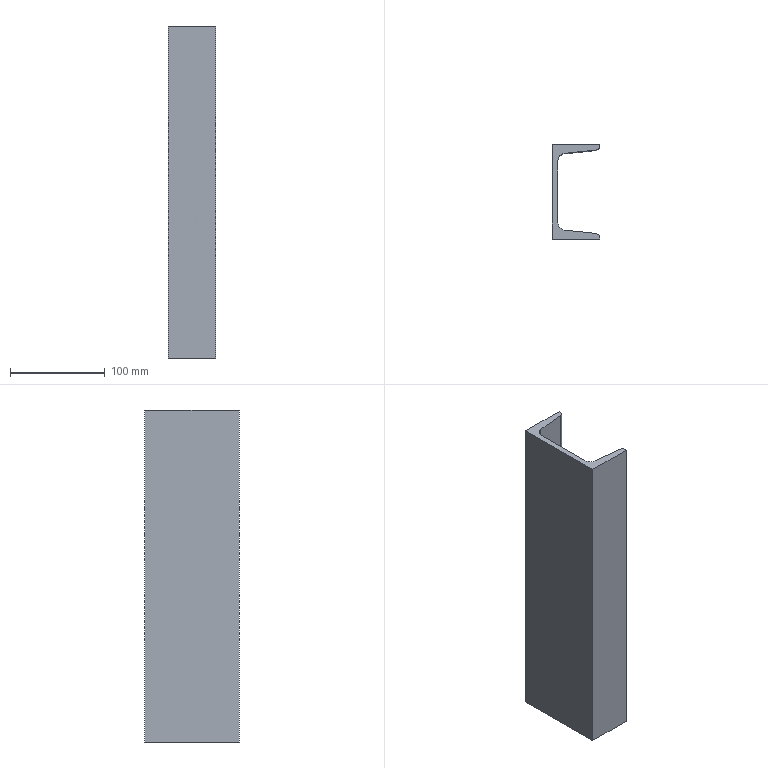Part | STEP file | ISO 657_11 CH 100 x 10 1784900428948 | 1 solid | 14 faces | box 50 x 100 x 350 mm | volume 458586 mm3 | plane 10 | cylinder 4 | commonest cylinder face diameters 9 x2 16 x2
STEP:
#1=CARTESIAN_POINT('',(4.39,-32.479,350.));
#2=VERTEX_POINT('',#1);
#3=CARTESIAN_POINT('',(11.554,-40.435,350.));
#4=VERTEX_POINT('',#3);
#5=CARTESIAN_POINT('',(12.39,-32.479,350.));
#6=DIRECTION('',(0.,0.,1.));
#7=DIRECTION('',(-1.,0.,0.));
#8=AXIS2_PLACEMENT_3D('',#5,#6,#7);
#9=CIRCLE('',#8,8.);
#10=EDGE_CURVE('',#2,#4,#9,.T.);
#11=ORIENTED_EDGE('',*,*,#10,.T.);
#12=CARTESIAN_POINT('',(11.554,-40.435,0.));
#13=VERTEX_POINT('',#12);
#14=CARTESIAN_POINT('',(11.554,-40.435,0.));
#15=DIRECTION('',(0.,0.,1.));
#16=VECTOR('',#15,10.);
#17=LINE('',#14,#16);
#18=EDGE_CURVE('',#13,#4,#17,.T.);
#19=ORIENTED_EDGE('',*,*,#18,.F.);
#20=CARTESIAN_POINT('',(4.39,-32.479,0.));
#21=VERTEX_POINT('',#20);
#22=CARTESIAN_POINT('',(12.39,-32.479,0.));
#23=DIRECTION('',(0.,0.,1.));
#24=DIRECTION('',(-1.,0.,0.));
#25=AXIS2_PLACEMENT_3D('',#22,#23,#24);
#26=CIRCLE('',#25,8.);
#27=EDGE_CURVE('',#21,#13,#26,.T.);
#28=ORIENTED_EDGE('',*,*,#27,.F.);
#29=CARTESIAN_POINT('',(4.39,-32.479,0.));
#30=DIRECTION('',(0.,0.,1.));
#31=VECTOR('',#30,10.);
#32=LINE('',#29,#31);
#33=EDGE_CURVE('',#21,#2,#32,.T.);
#34=ORIENTED_EDGE('',*,*,#33,.T.);
#35=EDGE_LOOP('',(#11,#19,#28,#34));
#36=FACE_OUTER_BOUND('',#35,.T.);
#37=CARTESIAN_POINT('',(12.39,-32.479,0.));
#38=DIRECTION('',(0.,0.,1.));
#39=DIRECTION('',(-1.,0.,0.));
#40=AXIS2_PLACEMENT_3D('',#37,#38,#39);
#41=CYLINDRICAL_SURFACE('',#40,8.);
#42=ADVANCED_FACE('',(#36),#41,.F.);
#43=CARTESIAN_POINT('',(44.46,-43.894,350.));
#44=VERTEX_POINT('',#43);
#45=CARTESIAN_POINT('',(15.355,-40.835,350.));
#46=DIRECTION('',(0.9945,-0.1045,0.));
#47=VECTOR('',#46,10.);
#48=LINE('',#45,#47);
#49=EDGE_CURVE('',#4,#44,#48,.T.);
#50=ORIENTED_EDGE('',*,*,#49,.T.);
#51=CARTESIAN_POINT('',(44.46,-43.894,0.));
#52=VERTEX_POINT('',#51);
#53=CARTESIAN_POINT('',(44.46,-43.894,0.));
#54=DIRECTION('',(0.,0.,1.));
#55=VECTOR('',#54,10.);
#56=LINE('',#53,#55);
#57=EDGE_CURVE('',#52,#44,#56,.T.);
#58=ORIENTED_EDGE('',*,*,#57,.F.);
#59=CARTESIAN_POINT('',(15.355,-40.835,0.));
#60=DIRECTION('',(0.9945,-0.1045,0.));
#61=VECTOR('',#60,10.);
#62=LINE('',#59,#61);
#63=EDGE_CURVE('',#13,#52,#62,.T.);
#64=ORIENTED_EDGE('',*,*,#63,.F.);
#65=ORIENTED_EDGE('',*,*,#18,.T.);
#66=EDGE_LOOP('',(#50,#58,#64,#65));
#67=FACE_OUTER_BOUND('',#66,.T.);
#68=CARTESIAN_POINT('',(11.554,-40.435,0.));
#69=DIRECTION('',(0.1045,0.9945,0.));
#70=DIRECTION('',(0.,0.,1.));
#71=AXIS2_PLACEMENT_3D('',#68,#69,#70);
#72=PLANE('',#71);
#73=ADVANCED_FACE('',(#67),#72,.T.);
#74=CARTESIAN_POINT('',(48.49,-48.369,350.));
#75=VERTEX_POINT('',#74);
#76=CARTESIAN_POINT('',(43.99,-48.369,350.));
#77=DIRECTION('',(0.,0.,-1.));
#78=DIRECTION('',(-1.,0.,0.));
#79=AXIS2_PLACEMENT_3D('',#76,#77,#78);
#80=CIRCLE('',#79,4.5);
#81=EDGE_CURVE('',#44,#75,#80,.T.);
#82=ORIENTED_EDGE('',*,*,#81,.T.);
#83=CARTESIAN_POINT('',(48.49,-48.369,0.));
#84=VERTEX_POINT('',#83);
#85=CARTESIAN_POINT('',(48.49,-48.369,0.));
#86=DIRECTION('',(0.,0.,1.));
#87=VECTOR('',#86,10.);
#88=LINE('',#85,#87);
#89=EDGE_CURVE('',#84,#75,#88,.T.);
#90=ORIENTED_EDGE('',*,*,#89,.F.);
#91=CARTESIAN_POINT('',(43.99,-48.369,0.));
#92=DIRECTION('',(0.,0.,-1.));
#93=DIRECTION('',(-1.,0.,0.));
#94=AXIS2_PLACEMENT_3D('',#91,#92,#93);
#95=CIRCLE('',#94,4.5);
#96=EDGE_CURVE('',#52,#84,#95,.T.);
#97=ORIENTED_EDGE('',*,*,#96,.F.);
#98=ORIENTED_EDGE('',*,*,#57,.T.);
#99=EDGE_LOOP('',(#82,#90,#97,#98));
#100=FACE_OUTER_BOUND('',#99,.T.);
#101=CARTESIAN_POINT('',(43.99,-48.369,0.));
#102=DIRECTION('',(0.,0.,1.));
#103=DIRECTION('',(-1.,0.,0.));
#104=AXIS2_PLACEMENT_3D('',#101,#102,#103);
#105=CYLINDRICAL_SURFACE('',#104,4.5);
#106=ADVANCED_FACE('',(#100),#105,.T.);
#107=CARTESIAN_POINT('',(48.49,-50.,350.));
#108=VERTEX_POINT('',#107);
#109=CARTESIAN_POINT('',(48.49,-24.185,350.));
#110=DIRECTION('',(0.,-1.,0.));
#111=VECTOR('',#110,10.);
#112=LINE('',#109,#111);
#113=EDGE_CURVE('',#75,#108,#112,.T.);
#114=ORIENTED_EDGE('',*,*,#113,.T.);
#115=CARTESIAN_POINT('',(48.49,-50.,0.));
#116=VERTEX_POINT('',#115);
#117=CARTESIAN_POINT('',(48.49,-50.,0.));
#118=DIRECTION('',(0.,0.,1.));
#119=VECTOR('',#118,10.);
#120=LINE('',#117,#119);
#121=EDGE_CURVE('',#116,#108,#120,.T.);
#122=ORIENTED_EDGE('',*,*,#121,.F.);
#123=CARTESIAN_POINT('',(48.49,-24.185,0.));
#124=DIRECTION('',(0.,-1.,0.));
#125=VECTOR('',#124,10.);
#126=LINE('',#123,#125);
#127=EDGE_CURVE('',#84,#116,#126,.T.);
#128=ORIENTED_EDGE('',*,*,#127,.F.);
#129=ORIENTED_EDGE('',*,*,#89,.T.);
#130=EDGE_LOOP('',(#114,#122,#128,#129));
#131=FACE_OUTER_BOUND('',#130,.T.);
#132=CARTESIAN_POINT('',(48.49,-48.369,0.));
#133=DIRECTION('',(1.,0.,0.));
#134=DIRECTION('',(0.,0.,-1.));
#135=AXIS2_PLACEMENT_3D('',#132,#133,#134);
#136=PLANE('',#135);
#137=ADVANCED_FACE('',(#131),#136,.T.);
#138=CARTESIAN_POINT('',(-1.51,-50.,350.));
#139=VERTEX_POINT('',#138);
#140=CARTESIAN_POINT('',(35.99,-50.,350.));
#141=DIRECTION('',(-1.,0.,0.));
#142=VECTOR('',#141,10.);
#143=LINE('',#140,#142);
#144=EDGE_CURVE('',#108,#139,#143,.T.);
#145=ORIENTED_EDGE('',*,*,#144,.T.);
#146=CARTESIAN_POINT('',(-1.51,-50.,0.));
#147=VERTEX_POINT('',#146);
#148=CARTESIAN_POINT('',(-1.51,-50.,0.));
#149=DIRECTION('',(0.,0.,1.));
#150=VECTOR('',#149,10.);
#151=LINE('',#148,#150);
#152=EDGE_CURVE('',#147,#139,#151,.T.);
#153=ORIENTED_EDGE('',*,*,#152,.F.);
#154=CARTESIAN_POINT('',(35.99,-50.,0.));
#155=DIRECTION('',(-1.,0.,0.));
#156=VECTOR('',#155,10.);
#157=LINE('',#154,#156);
#158=EDGE_CURVE('',#116,#147,#157,.T.);
#159=ORIENTED_EDGE('',*,*,#158,.F.);
#160=ORIENTED_EDGE('',*,*,#121,.T.);
#161=EDGE_LOOP('',(#145,#153,#159,#160));
#162=FACE_OUTER_BOUND('',#161,.T.);
#163=CARTESIAN_POINT('',(48.49,-50.,0.));
#164=DIRECTION('',(0.,-1.,0.));
#165=DIRECTION('',(0.,0.,-1.));
#166=AXIS2_PLACEMENT_3D('',#163,#164,#165);
#167=PLANE('',#166);
#168=ADVANCED_FACE('',(#162),#167,.T.);
#169=CARTESIAN_POINT('',(-1.51,50.,350.));
#170=VERTEX_POINT('',#169);
#171=CARTESIAN_POINT('',(-1.51,0.,350.));
#172=DIRECTION('',(0.,1.,0.));
#173=VECTOR('',#172,10.);
#174=LINE('',#171,#173);
#175=EDGE_CURVE('',#139,#170,#174,.T.);
#176=ORIENTED_EDGE('',*,*,#175,.T.);
#177=CARTESIAN_POINT('',(-1.51,50.,0.));
#178=VERTEX_POINT('',#177);
#179=CARTESIAN_POINT('',(-1.51,50.,0.));
#180=DIRECTION('',(0.,0.,1.));
#181=VECTOR('',#180,10.);
#182=LINE('',#179,#181);
#183=EDGE_CURVE('',#178,#170,#182,.T.);
#184=ORIENTED_EDGE('',*,*,#183,.F.);
#185=CARTESIAN_POINT('',(-1.51,0.,0.));
#186=DIRECTION('',(0.,1.,0.));
#187=VECTOR('',#186,10.);
#188=LINE('',#185,#187);
#189=EDGE_CURVE('',#147,#178,#188,.T.);
#190=ORIENTED_EDGE('',*,*,#189,.F.);
#191=ORIENTED_EDGE('',*,*,#152,.T.);
#192=EDGE_LOOP('',(#176,#184,#190,#191));
#193=FACE_OUTER_BOUND('',#192,.T.);
#194=CARTESIAN_POINT('',(-1.51,0.,0.));
#195=DIRECTION('',(-1.,0.,0.));
#196=DIRECTION('',(0.,0.,1.));
#197=AXIS2_PLACEMENT_3D('',#194,#195,#196);
#198=PLANE('',#197);
#199=ADVANCED_FACE('',(#193),#198,.T.);
#200=CARTESIAN_POINT('',(48.49,50.,350.));
#201=VERTEX_POINT('',#200);
#202=CARTESIAN_POINT('',(10.99,50.,350.));
#203=DIRECTION('',(1.,0.,0.));
#204=VECTOR('',#203,10.);
#205=LINE('',#202,#204);
#206=EDGE_CURVE('',#170,#201,#205,.T.);
#207=ORIENTED_EDGE('',*,*,#206,.T.);
#208=CARTESIAN_POINT('',(48.49,50.,0.));
#209=VERTEX_POINT('',#208);
#210=CARTESIAN_POINT('',(48.49,50.,0.));
#211=DIRECTION('',(0.,0.,1.));
#212=VECTOR('',#211,10.);
#213=LINE('',#210,#212);
#214=EDGE_CURVE('',#209,#201,#213,.T.);
#215=ORIENTED_EDGE('',*,*,#214,.F.);
#216=CARTESIAN_POINT('',(10.99,50.,0.));
#217=DIRECTION('',(1.,0.,0.));
#218=VECTOR('',#217,10.);
#219=LINE('',#216,#218);
#220=EDGE_CURVE('',#178,#209,#219,.T.);
#221=ORIENTED_EDGE('',*,*,#220,.F.);
#222=ORIENTED_EDGE('',*,*,#183,.T.);
#223=EDGE_LOOP('',(#207,#215,#221,#222));
#224=FACE_OUTER_BOUND('',#223,.T.);
#225=CARTESIAN_POINT('',(-1.51,50.,0.));
#226=DIRECTION('',(0.,1.,0.));
#227=DIRECTION('',(0.,0.,1.));
#228=AXIS2_PLACEMENT_3D('',#225,#226,#227);
#229=PLANE('',#228);
#230=ADVANCED_FACE('',(#224),#229,.T.);
#231=CARTESIAN_POINT('',(48.49,48.369,350.));
#232=VERTEX_POINT('',#231);
#233=CARTESIAN_POINT('',(48.49,25.,350.));
#234=DIRECTION('',(0.,-1.,0.));
#235=VECTOR('',#234,10.);
#236=LINE('',#233,#235);
#237=EDGE_CURVE('',#201,#232,#236,.T.);
#238=ORIENTED_EDGE('',*,*,#237,.T.);
#239=CARTESIAN_POINT('',(48.49,48.369,0.));
#240=VERTEX_POINT('',#239);
#241=CARTESIAN_POINT('',(48.49,48.369,0.));
#242=DIRECTION('',(0.,0.,1.));
#243=VECTOR('',#242,10.);
#244=LINE('',#241,#243);
#245=EDGE_CURVE('',#240,#232,#244,.T.);
#246=ORIENTED_EDGE('',*,*,#245,.F.);
#247=CARTESIAN_POINT('',(48.49,25.,0.));
#248=DIRECTION('',(0.,-1.,0.));
#249=VECTOR('',#248,10.);
#250=LINE('',#247,#249);
#251=EDGE_CURVE('',#209,#240,#250,.T.);
#252=ORIENTED_EDGE('',*,*,#251,.F.);
#253=ORIENTED_EDGE('',*,*,#214,.T.);
#254=EDGE_LOOP('',(#238,#246,#252,#253));
#255=FACE_OUTER_BOUND('',#254,.T.);
#256=CARTESIAN_POINT('',(48.49,50.,0.));
#257=DIRECTION('',(1.,0.,0.));
#258=DIRECTION('',(0.,0.,-1.));
#259=AXIS2_PLACEMENT_3D('',#256,#257,#258);
#260=PLANE('',#259);
#261=ADVANCED_FACE('',(#255),#260,.T.);
#262=CARTESIAN_POINT('',(44.46,43.894,350.));
#263=VERTEX_POINT('',#262);
#264=CARTESIAN_POINT('',(43.99,48.369,350.));
#265=DIRECTION('',(0.,0.,-1.));
#266=DIRECTION('',(-0.1045,0.9945,0.));
#267=AXIS2_PLACEMENT_3D('',#264,#265,#266);
#268=CIRCLE('',#267,4.5);
#269=EDGE_CURVE('',#232,#263,#268,.T.);
#270=ORIENTED_EDGE('',*,*,#269,.T.);
#271=CARTESIAN_POINT('',(44.46,43.894,0.));
#272=VERTEX_POINT('',#271);
#273=CARTESIAN_POINT('',(44.46,43.894,0.));
#274=DIRECTION('',(0.,0.,1.));
#275=VECTOR('',#274,10.);
#276=LINE('',#273,#275);
#277=EDGE_CURVE('',#272,#263,#276,.T.);
#278=ORIENTED_EDGE('',*,*,#277,.F.);
#279=CARTESIAN_POINT('',(43.99,48.369,0.));
#280=DIRECTION('',(0.,0.,-1.));
#281=DIRECTION('',(-0.1045,0.9945,0.));
#282=AXIS2_PLACEMENT_3D('',#279,#280,#281);
#283=CIRCLE('',#282,4.5);
#284=EDGE_CURVE('',#240,#272,#283,.T.);
#285=ORIENTED_EDGE('',*,*,#284,.F.);
#286=ORIENTED_EDGE('',*,*,#245,.T.);
#287=EDGE_LOOP('',(#270,#278,#285,#286));
#288=FACE_OUTER_BOUND('',#287,.T.);
#289=CARTESIAN_POINT('',(43.99,48.369,0.));
#290=DIRECTION('',(0.,0.,1.));
#291=DIRECTION('',(-0.1045,0.9945,0.));
#292=AXIS2_PLACEMENT_3D('',#289,#290,#291);
#293=CYLINDRICAL_SURFACE('',#292,4.5);
#294=ADVANCED_FACE('',(#288),#293,.T.);
#295=CARTESIAN_POINT('',(11.554,40.435,350.));
#296=VERTEX_POINT('',#295);
#297=CARTESIAN_POINT('',(31.808,42.564,350.));
#298=DIRECTION('',(-0.9945,-0.1045,0.));
#299=VECTOR('',#298,10.);
#300=LINE('',#297,#299);
#301=EDGE_CURVE('',#263,#296,#300,.T.);
#302=ORIENTED_EDGE('',*,*,#301,.T.);
#303=CARTESIAN_POINT('',(11.554,40.435,0.));
#304=VERTEX_POINT('',#303);
#305=CARTESIAN_POINT('',(11.554,40.435,0.));
#306=DIRECTION('',(0.,0.,1.));
#307=VECTOR('',#306,10.);
#308=LINE('',#305,#307);
#309=EDGE_CURVE('',#304,#296,#308,.T.);
#310=ORIENTED_EDGE('',*,*,#309,.F.);
#311=CARTESIAN_POINT('',(31.808,42.564,0.));
#312=DIRECTION('',(-0.9945,-0.1045,0.));
#313=VECTOR('',#312,10.);
#314=LINE('',#311,#313);
#315=EDGE_CURVE('',#272,#304,#314,.T.);
#316=ORIENTED_EDGE('',*,*,#315,.F.);
#317=ORIENTED_EDGE('',*,*,#277,.T.);
#318=EDGE_LOOP('',(#302,#310,#316,#317));
#319=FACE_OUTER_BOUND('',#318,.T.);
#320=CARTESIAN_POINT('',(44.46,43.894,0.));
#321=DIRECTION('',(0.1045,-0.9945,0.));
#322=DIRECTION('',(0.,0.,-1.));
#323=AXIS2_PLACEMENT_3D('',#320,#321,#322);
#324=PLANE('',#323);
#325=ADVANCED_FACE('',(#319),#324,.T.);
#326=CARTESIAN_POINT('',(4.39,32.479,350.));
#327=VERTEX_POINT('',#326);
#328=CARTESIAN_POINT('',(12.39,32.479,350.));
#329=DIRECTION('',(0.,0.,1.));
#330=DIRECTION('',(-0.1045,0.9945,0.));
#331=AXIS2_PLACEMENT_3D('',#328,#329,#330);
#332=CIRCLE('',#331,8.);
#333=EDGE_CURVE('',#296,#327,#332,.T.);
#334=ORIENTED_EDGE('',*,*,#333,.T.);
#335=CARTESIAN_POINT('',(4.39,32.479,0.));
#336=VERTEX_POINT('',#335);
#337=CARTESIAN_POINT('',(4.39,32.479,0.));
#338=DIRECTION('',(0.,0.,1.));
#339=VECTOR('',#338,10.);
#340=LINE('',#337,#339);
#341=EDGE_CURVE('',#336,#327,#340,.T.);
#342=ORIENTED_EDGE('',*,*,#341,.F.);
#343=CARTESIAN_POINT('',(12.39,32.479,0.));
#344=DIRECTION('',(0.,0.,1.));
#345=DIRECTION('',(-0.1045,0.9945,0.));
#346=AXIS2_PLACEMENT_3D('',#343,#344,#345);
#347=CIRCLE('',#346,8.);
#348=EDGE_CURVE('',#304,#336,#347,.T.);
#349=ORIENTED_EDGE('',*,*,#348,.F.);
#350=ORIENTED_EDGE('',*,*,#309,.T.);
#351=EDGE_LOOP('',(#334,#342,#349,#350));
#352=FACE_OUTER_BOUND('',#351,.T.);
#353=CARTESIAN_POINT('',(12.39,32.479,0.));
#354=DIRECTION('',(0.,0.,1.));
#355=DIRECTION('',(-0.1045,0.9945,0.));
#356=AXIS2_PLACEMENT_3D('',#353,#354,#355);
#357=CYLINDRICAL_SURFACE('',#356,8.);
#358=ADVANCED_FACE('',(#352),#357,.F.);
#359=CARTESIAN_POINT('',(4.39,0.,350.));
#360=DIRECTION('',(0.,-1.,0.));
#361=VECTOR('',#360,10.);
#362=LINE('',#359,#361);
#363=EDGE_CURVE('',#327,#2,#362,.T.);
#364=ORIENTED_EDGE('',*,*,#363,.T.);
#365=ORIENTED_EDGE('',*,*,#33,.F.);
#366=CARTESIAN_POINT('',(4.39,0.,0.));
#367=DIRECTION('',(0.,-1.,0.));
#368=VECTOR('',#367,10.);
#369=LINE('',#366,#368);
#370=EDGE_CURVE('',#336,#21,#369,.T.);
#371=ORIENTED_EDGE('',*,*,#370,.F.);
#372=ORIENTED_EDGE('',*,*,#341,.T.);
#373=EDGE_LOOP('',(#364,#365,#371,#372));
#374=FACE_OUTER_BOUND('',#373,.T.);
#375=CARTESIAN_POINT('',(4.39,0.,0.));
#376=DIRECTION('',(1.,0.,0.));
#377=DIRECTION('',(0.,0.,-1.));
#378=AXIS2_PLACEMENT_3D('',#375,#376,#377);
#379=PLANE('',#378);
#380=ADVANCED_FACE('',(#374),#379,.T.);
#381=ORIENTED_EDGE('',*,*,#220,.T.);
#382=ORIENTED_EDGE('',*,*,#251,.T.);
#383=ORIENTED_EDGE('',*,*,#284,.T.);
#384=ORIENTED_EDGE('',*,*,#315,.T.);
#385=ORIENTED_EDGE('',*,*,#348,.T.);
#386=ORIENTED_EDGE('',*,*,#370,.T.);
#387=ORIENTED_EDGE('',*,*,#27,.T.);
#388=ORIENTED_EDGE('',*,*,#63,.T.);
#389=ORIENTED_EDGE('',*,*,#96,.T.);
#390=ORIENTED_EDGE('',*,*,#127,.T.);
#391=ORIENTED_EDGE('',*,*,#158,.T.);
#392=ORIENTED_EDGE('',*,*,#189,.T.);
#393=EDGE_LOOP('',(#381,#382,#383,#384,#385,#386,#387,#388,#389,#390,#391,#392));
#394=FACE_OUTER_BOUND('',#393,.T.);
#395=CARTESIAN_POINT('',(23.49,0.,0.));
#396=DIRECTION('',(0.,0.,1.));
#397=DIRECTION('',(1.,0.,0.));
#398=AXIS2_PLACEMENT_3D('',#395,#396,#397);
#399=PLANE('',#398);
#400=ADVANCED_FACE('',(#394),#399,.F.);
#401=ORIENTED_EDGE('',*,*,#206,.F.);
#402=ORIENTED_EDGE('',*,*,#175,.F.);
#403=ORIENTED_EDGE('',*,*,#144,.F.);
#404=ORIENTED_EDGE('',*,*,#113,.F.);
#405=ORIENTED_EDGE('',*,*,#81,.F.);
#406=ORIENTED_EDGE('',*,*,#49,.F.);
#407=ORIENTED_EDGE('',*,*,#10,.F.);
#408=ORIENTED_EDGE('',*,*,#363,.F.);
#409=ORIENTED_EDGE('',*,*,#333,.F.);
#410=ORIENTED_EDGE('',*,*,#301,.F.);
#411=ORIENTED_EDGE('',*,*,#269,.F.);
#412=ORIENTED_EDGE('',*,*,#237,.F.);
#413=EDGE_LOOP('',(#401,#402,#403,#404,#405,#406,#407,#408,#409,#410,#411,#412));
#414=FACE_OUTER_BOUND('',#413,.T.);
#415=CARTESIAN_POINT('',(23.49,0.,350.));
#416=DIRECTION('',(0.,0.,1.));
#417=DIRECTION('',(1.,0.,0.));
#418=AXIS2_PLACEMENT_3D('',#415,#416,#417);
#419=PLANE('',#418);
#420=ADVANCED_FACE('',(#414),#419,.T.);
#421=CLOSED_SHELL('',(#42,#73,#106,#137,#168,#199,#230,#261,#294,#325,#358,#380,#400,#420));
#422=MANIFOLD_SOLID_BREP('',#421);
#423=(LENGTH_UNIT()NAMED_UNIT(*)SI_UNIT(.MILLI.,.METRE.));
#424=UNCERTAINTY_MEASURE_WITH_UNIT(LENGTH_MEASURE(0.01),#423,'','');
#425=(NAMED_UNIT(*)PLANE_ANGLE_UNIT()SI_UNIT($,.RADIAN.));
#426=(NAMED_UNIT(*)SI_UNIT($,.STERADIAN.)SOLID_ANGLE_UNIT());
#427=(GEOMETRIC_REPRESENTATION_CONTEXT(3)GLOBAL_UNCERTAINTY_ASSIGNED_CONTEXT((#424))GLOBAL_UNIT_ASSIGNED_CONTEXT((#423,#425,#426))REPRESENTATION_CONTEXT('',''));
#428=ADVANCED_BREP_SHAPE_REPRESENTATION('',(#422),#427);